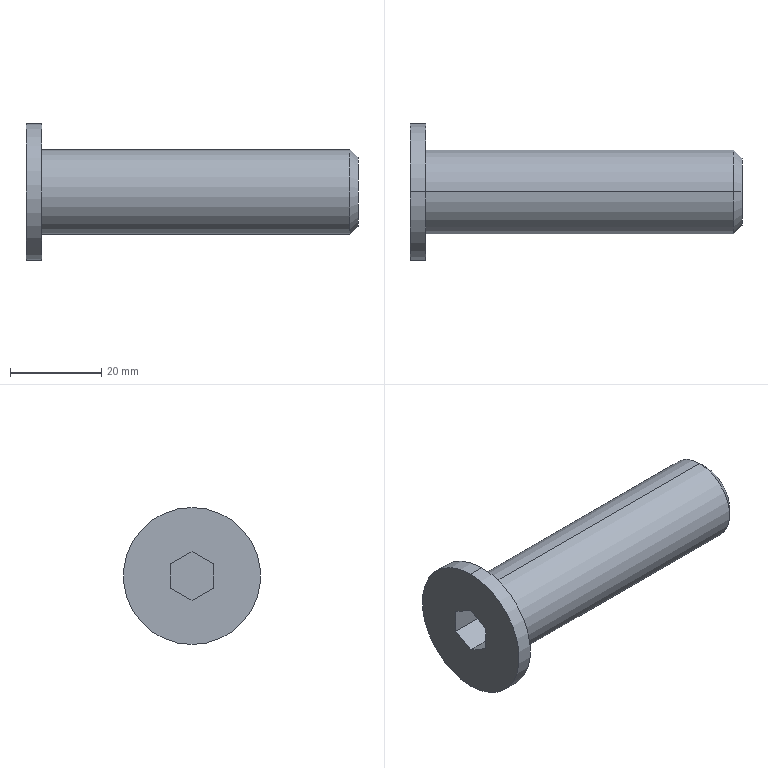Part | SolidWorks | features BaseBody 1 | 1 solid | 16 faces | box 72.692 x 30 x 30 mm | volume 20042 mm3 | plane 10 | cylinder 4 | cone 2 | commonest cylinder face diameters 18.462 x2 30 x2
STEP:
#1=CARTESIAN_POINT('',(-37.408,269.115,278.462));
#2=VERTEX_POINT('',#1);
#3=CARTESIAN_POINT('',(-37.408,269.115,260.));
#4=VERTEX_POINT('',#3);
#5=CARTESIAN_POINT('',(-37.408,269.115,269.231));
#6=DIRECTION('',(-1.,0.,0.));
#7=DIRECTION('',(0.,0.,1.));
#8=AXIS2_PLACEMENT_3D('',#5,#6,#7);
#9=CIRCLE('',#8,9.231);
#10=EDGE_CURVE('',#2,#4,#9,.T.);
#11=ORIENTED_EDGE('',*,*,#10,.T.);
#12=CARTESIAN_POINT('',(-104.869,269.115,260.));
#13=VERTEX_POINT('',#12);
#14=CARTESIAN_POINT('',(-35.638,269.115,260.));
#15=DIRECTION('',(-1.,0.,0.));
#16=VECTOR('',#15,1000.);
#17=LINE('',#14,#16);
#18=EDGE_CURVE('',#4,#13,#17,.T.);
#19=ORIENTED_EDGE('',*,*,#18,.T.);
#20=CARTESIAN_POINT('',(-104.869,269.115,278.462));
#21=VERTEX_POINT('',#20);
#22=CARTESIAN_POINT('',(-104.869,269.115,269.231));
#23=DIRECTION('',(1.,0.,0.));
#24=DIRECTION('',(0.,0.,1.));
#25=AXIS2_PLACEMENT_3D('',#22,#23,#24);
#26=CIRCLE('',#25,9.231);
#27=EDGE_CURVE('',#13,#21,#26,.T.);
#28=ORIENTED_EDGE('',*,*,#27,.T.);
#29=CARTESIAN_POINT('',(-35.638,269.115,278.462));
#30=DIRECTION('',(-1.,0.,0.));
#31=VECTOR('',#30,1000.);
#32=LINE('',#29,#31);
#33=EDGE_CURVE('',#2,#21,#32,.T.);
#34=ORIENTED_EDGE('',*,*,#33,.F.);
#35=EDGE_LOOP('',(#11,#19,#28,#34));
#36=FACE_OUTER_BOUND('',#35,.T.);
#37=CARTESIAN_POINT('',(-35.638,269.115,269.231));
#38=DIRECTION('',(-1.,0.,0.));
#39=DIRECTION('',(0.,0.,1.));
#40=AXIS2_PLACEMENT_3D('',#37,#38,#39);
#41=CYLINDRICAL_SURFACE('',#40,9.231);
#42=ADVANCED_FACE('',(#36),#41,.T.);
#43=CARTESIAN_POINT('',(-35.638,269.115,276.692));
#44=VERTEX_POINT('',#43);
#45=CARTESIAN_POINT('',(-35.638,269.115,261.77));
#46=VERTEX_POINT('',#45);
#47=CARTESIAN_POINT('',(-35.638,269.115,269.231));
#48=DIRECTION('',(-1.,0.,0.));
#49=DIRECTION('',(0.,0.,1.));
#50=AXIS2_PLACEMENT_3D('',#47,#48,#49);
#51=CIRCLE('',#50,7.461);
#52=EDGE_CURVE('',#44,#46,#51,.T.);
#53=ORIENTED_EDGE('',*,*,#52,.T.);
#54=CARTESIAN_POINT('',(-37.408,269.115,260.));
#55=DIRECTION('',(-0.7071,0.,-0.7071));
#56=VECTOR('',#55,1000.);
#57=LINE('',#54,#56);
#58=EDGE_CURVE('',#46,#4,#57,.T.);
#59=ORIENTED_EDGE('',*,*,#58,.T.);
#60=ORIENTED_EDGE('',*,*,#10,.F.);
#61=CARTESIAN_POINT('',(-37.408,269.115,278.462));
#62=DIRECTION('',(-0.7071,0.,0.7071));
#63=VECTOR('',#62,1000.);
#64=LINE('',#61,#63);
#65=EDGE_CURVE('',#44,#2,#64,.T.);
#66=ORIENTED_EDGE('',*,*,#65,.F.);
#67=EDGE_LOOP('',(#53,#59,#60,#66));
#68=FACE_OUTER_BOUND('',#67,.T.);
#69=CARTESIAN_POINT('',(-37.408,269.115,269.231));
#70=DIRECTION('',(-1.,0.,0.));
#71=DIRECTION('',(0.,0.,1.));
#72=AXIS2_PLACEMENT_3D('',#69,#70,#71);
#73=CONICAL_SURFACE('',#72,9.231,0.7854);
#74=ADVANCED_FACE('',(#68),#73,.T.);
#75=CARTESIAN_POINT('',(-104.869,269.115,284.231));
#76=VERTEX_POINT('',#75);
#77=CARTESIAN_POINT('',(-104.869,269.115,254.231));
#78=VERTEX_POINT('',#77);
#79=CARTESIAN_POINT('',(-104.869,269.115,269.231));
#80=DIRECTION('',(-1.,0.,0.));
#81=DIRECTION('',(0.,0.,1.));
#82=AXIS2_PLACEMENT_3D('',#79,#80,#81);
#83=CIRCLE('',#82,15.);
#84=EDGE_CURVE('',#76,#78,#83,.T.);
#85=ORIENTED_EDGE('',*,*,#84,.T.);
#86=CARTESIAN_POINT('',(-108.33,269.115,254.231));
#87=VERTEX_POINT('',#86);
#88=CARTESIAN_POINT('',(-35.638,269.115,254.231));
#89=DIRECTION('',(-1.,0.,0.));
#90=VECTOR('',#89,1000.);
#91=LINE('',#88,#90);
#92=EDGE_CURVE('',#78,#87,#91,.T.);
#93=ORIENTED_EDGE('',*,*,#92,.T.);
#94=CARTESIAN_POINT('',(-108.33,269.115,284.231));
#95=VERTEX_POINT('',#94);
#96=CARTESIAN_POINT('',(-108.33,269.115,269.231));
#97=DIRECTION('',(1.,0.,0.));
#98=DIRECTION('',(0.,0.,1.));
#99=AXIS2_PLACEMENT_3D('',#96,#97,#98);
#100=CIRCLE('',#99,15.);
#101=EDGE_CURVE('',#87,#95,#100,.T.);
#102=ORIENTED_EDGE('',*,*,#101,.T.);
#103=CARTESIAN_POINT('',(-35.638,269.115,284.231));
#104=DIRECTION('',(-1.,0.,0.));
#105=VECTOR('',#104,1000.);
#106=LINE('',#103,#105);
#107=EDGE_CURVE('',#76,#95,#106,.T.);
#108=ORIENTED_EDGE('',*,*,#107,.F.);
#109=EDGE_LOOP('',(#85,#93,#102,#108));
#110=FACE_OUTER_BOUND('',#109,.T.);
#111=CARTESIAN_POINT('',(-35.638,269.115,269.231));
#112=DIRECTION('',(-1.,0.,0.));
#113=DIRECTION('',(0.,0.,1.));
#114=AXIS2_PLACEMENT_3D('',#111,#112,#113);
#115=CYLINDRICAL_SURFACE('',#114,15.);
#116=ADVANCED_FACE('',(#110),#115,.T.);
#117=ORIENTED_EDGE('',*,*,#18,.F.);
#118=CARTESIAN_POINT('',(-37.408,269.115,269.231));
#119=DIRECTION('',(-1.,0.,0.));
#120=DIRECTION('',(0.,0.,1.));
#121=AXIS2_PLACEMENT_3D('',#118,#119,#120);
#122=CIRCLE('',#121,9.231);
#123=EDGE_CURVE('',#4,#2,#122,.T.);
#124=ORIENTED_EDGE('',*,*,#123,.T.);
#125=ORIENTED_EDGE('',*,*,#33,.T.);
#126=CARTESIAN_POINT('',(-104.869,269.115,269.231));
#127=DIRECTION('',(1.,0.,0.));
#128=DIRECTION('',(0.,0.,1.));
#129=AXIS2_PLACEMENT_3D('',#126,#127,#128);
#130=CIRCLE('',#129,9.231);
#131=EDGE_CURVE('',#21,#13,#130,.T.);
#132=ORIENTED_EDGE('',*,*,#131,.T.);
#133=EDGE_LOOP('',(#117,#124,#125,#132));
#134=FACE_OUTER_BOUND('',#133,.T.);
#135=CARTESIAN_POINT('',(-35.638,269.115,269.231));
#136=DIRECTION('',(-1.,0.,0.));
#137=DIRECTION('',(0.,0.,1.));
#138=AXIS2_PLACEMENT_3D('',#135,#136,#137);
#139=CYLINDRICAL_SURFACE('',#138,9.231);
#140=ADVANCED_FACE('',(#134),#139,.T.);
#141=ORIENTED_EDGE('',*,*,#58,.F.);
#142=CARTESIAN_POINT('',(-35.638,269.115,269.231));
#143=DIRECTION('',(-1.,0.,0.));
#144=DIRECTION('',(0.,0.,1.));
#145=AXIS2_PLACEMENT_3D('',#142,#143,#144);
#146=CIRCLE('',#145,7.461);
#147=EDGE_CURVE('',#46,#44,#146,.T.);
#148=ORIENTED_EDGE('',*,*,#147,.T.);
#149=ORIENTED_EDGE('',*,*,#65,.T.);
#150=ORIENTED_EDGE('',*,*,#123,.F.);
#151=EDGE_LOOP('',(#141,#148,#149,#150));
#152=FACE_OUTER_BOUND('',#151,.T.);
#153=CARTESIAN_POINT('',(-37.408,269.115,269.231));
#154=DIRECTION('',(-1.,0.,0.));
#155=DIRECTION('',(0.,0.,1.));
#156=AXIS2_PLACEMENT_3D('',#153,#154,#155);
#157=CONICAL_SURFACE('',#156,9.231,0.7854);
#158=ADVANCED_FACE('',(#152),#157,.T.);
#159=ORIENTED_EDGE('',*,*,#131,.F.);
#160=ORIENTED_EDGE('',*,*,#27,.F.);
#161=EDGE_LOOP('',(#159,#160));
#162=FACE_BOUND('',#161,.T.);
#163=ORIENTED_EDGE('',*,*,#84,.F.);
#164=CARTESIAN_POINT('',(-104.869,269.115,269.231));
#165=DIRECTION('',(-1.,0.,0.));
#166=DIRECTION('',(0.,0.,1.));
#167=AXIS2_PLACEMENT_3D('',#164,#165,#166);
#168=CIRCLE('',#167,15.);
#169=EDGE_CURVE('',#78,#76,#168,.T.);
#170=ORIENTED_EDGE('',*,*,#169,.F.);
#171=EDGE_LOOP('',(#163,#170));
#172=FACE_OUTER_BOUND('',#171,.T.);
#173=CARTESIAN_POINT('',(-104.869,284.115,269.231));
#174=DIRECTION('',(-1.,0.,0.));
#175=DIRECTION('',(0.,0.,1.));
#176=AXIS2_PLACEMENT_3D('',#173,#174,#175);
#177=PLANE('',#176);
#178=ADVANCED_FACE('',(#162,#172),#177,.F.);
#179=ORIENTED_EDGE('',*,*,#52,.F.);
#180=ORIENTED_EDGE('',*,*,#147,.F.);
#181=EDGE_LOOP('',(#179,#180));
#182=FACE_OUTER_BOUND('',#181,.T.);
#183=CARTESIAN_POINT('',(-35.638,276.576,269.231));
#184=DIRECTION('',(-1.,0.,0.));
#185=DIRECTION('',(0.,0.,1.));
#186=AXIS2_PLACEMENT_3D('',#183,#184,#185);
#187=PLANE('',#186);
#188=ADVANCED_FACE('',(#182),#187,.F.);
#189=ORIENTED_EDGE('',*,*,#92,.F.);
#190=ORIENTED_EDGE('',*,*,#169,.T.);
#191=ORIENTED_EDGE('',*,*,#107,.T.);
#192=CARTESIAN_POINT('',(-108.33,269.115,269.231));
#193=DIRECTION('',(1.,0.,0.));
#194=DIRECTION('',(0.,0.,1.));
#195=AXIS2_PLACEMENT_3D('',#192,#193,#194);
#196=CIRCLE('',#195,15.);
#197=EDGE_CURVE('',#95,#87,#196,.T.);
#198=ORIENTED_EDGE('',*,*,#197,.T.);
#199=EDGE_LOOP('',(#189,#190,#191,#198));
#200=FACE_OUTER_BOUND('',#199,.T.);
#201=CARTESIAN_POINT('',(-35.638,269.115,269.231));
#202=DIRECTION('',(-1.,0.,0.));
#203=DIRECTION('',(0.,0.,1.));
#204=AXIS2_PLACEMENT_3D('',#201,#202,#203);
#205=CYLINDRICAL_SURFACE('',#204,15.);
#206=ADVANCED_FACE('',(#200),#205,.T.);
#207=CARTESIAN_POINT('',(-108.33,273.731,271.895));
#208=VERTEX_POINT('',#207);
#209=CARTESIAN_POINT('',(-108.33,273.731,266.566));
#210=VERTEX_POINT('',#209);
#211=CARTESIAN_POINT('',(-108.33,273.731,269.231));
#212=DIRECTION('',(0.,0.,-1.));
#213=VECTOR('',#212,1000.);
#214=LINE('',#211,#213);
#215=EDGE_CURVE('',#208,#210,#214,.T.);
#216=ORIENTED_EDGE('',*,*,#215,.F.);
#217=CARTESIAN_POINT('',(-108.33,269.115,274.56));
#218=VERTEX_POINT('',#217);
#219=CARTESIAN_POINT('',(-108.33,269.115,274.56));
#220=DIRECTION('',(0.,0.866,-0.5));
#221=VECTOR('',#220,1000.);
#222=LINE('',#219,#221);
#223=EDGE_CURVE('',#218,#208,#222,.T.);
#224=ORIENTED_EDGE('',*,*,#223,.F.);
#225=CARTESIAN_POINT('',(-108.33,264.5,271.895));
#226=VERTEX_POINT('',#225);
#227=CARTESIAN_POINT('',(-108.33,264.5,271.895));
#228=DIRECTION('',(0.,0.866,0.5));
#229=VECTOR('',#228,1000.);
#230=LINE('',#227,#229);
#231=EDGE_CURVE('',#226,#218,#230,.T.);
#232=ORIENTED_EDGE('',*,*,#231,.F.);
#233=CARTESIAN_POINT('',(-108.33,264.5,266.566));
#234=VERTEX_POINT('',#233);
#235=CARTESIAN_POINT('',(-108.33,264.5,269.231));
#236=DIRECTION('',(0.,0.,1.));
#237=VECTOR('',#236,1000.);
#238=LINE('',#235,#237);
#239=EDGE_CURVE('',#234,#226,#238,.T.);
#240=ORIENTED_EDGE('',*,*,#239,.F.);
#241=CARTESIAN_POINT('',(-108.33,269.115,263.901));
#242=VERTEX_POINT('',#241);
#243=CARTESIAN_POINT('',(-108.33,269.115,263.901));
#244=DIRECTION('',(0.,-0.866,0.5));
#245=VECTOR('',#244,1000.);
#246=LINE('',#243,#245);
#247=EDGE_CURVE('',#242,#234,#246,.T.);
#248=ORIENTED_EDGE('',*,*,#247,.F.);
#249=CARTESIAN_POINT('',(-108.33,273.731,266.566));
#250=DIRECTION('',(0.,-0.866,-0.5));
#251=VECTOR('',#250,1000.);
#252=LINE('',#249,#251);
#253=EDGE_CURVE('',#210,#242,#252,.T.);
#254=ORIENTED_EDGE('',*,*,#253,.F.);
#255=EDGE_LOOP('',(#216,#224,#232,#240,#248,#254));
#256=FACE_BOUND('',#255,.T.);
#257=ORIENTED_EDGE('',*,*,#197,.F.);
#258=ORIENTED_EDGE('',*,*,#101,.F.);
#259=EDGE_LOOP('',(#257,#258));
#260=FACE_OUTER_BOUND('',#259,.T.);
#261=CARTESIAN_POINT('',(-108.33,269.115,269.231));
#262=DIRECTION('',(1.,0.,0.));
#263=DIRECTION('',(0.,0.,-1.));
#264=AXIS2_PLACEMENT_3D('',#261,#262,#263);
#265=PLANE('',#264);
#266=ADVANCED_FACE('',(#256,#260),#265,.F.);
#267=CARTESIAN_POINT('',(-96.792,269.115,263.901));
#268=VERTEX_POINT('',#267);
#269=CARTESIAN_POINT('',(-96.792,269.115,263.901));
#270=DIRECTION('',(1.,0.,0.));
#271=VECTOR('',#270,1000.);
#272=LINE('',#269,#271);
#273=EDGE_CURVE('',#242,#268,#272,.T.);
#274=ORIENTED_EDGE('',*,*,#273,.T.);
#275=CARTESIAN_POINT('',(-96.792,273.731,266.566));
#276=VERTEX_POINT('',#275);
#277=CARTESIAN_POINT('',(-96.792,269.115,263.901));
#278=DIRECTION('',(0.,0.866,0.5));
#279=VECTOR('',#278,1000.);
#280=LINE('',#277,#279);
#281=EDGE_CURVE('',#268,#276,#280,.T.);
#282=ORIENTED_EDGE('',*,*,#281,.T.);
#283=CARTESIAN_POINT('',(-96.792,273.731,266.566));
#284=DIRECTION('',(-1.,0.,0.));
#285=VECTOR('',#284,1000.);
#286=LINE('',#283,#285);
#287=EDGE_CURVE('',#276,#210,#286,.T.);
#288=ORIENTED_EDGE('',*,*,#287,.T.);
#289=ORIENTED_EDGE('',*,*,#253,.T.);
#290=EDGE_LOOP('',(#274,#282,#288,#289));
#291=FACE_OUTER_BOUND('',#290,.T.);
#292=CARTESIAN_POINT('',(-96.792,269.115,263.901));
#293=DIRECTION('',(0.,-0.5,0.866));
#294=DIRECTION('',(0.,-0.866,-0.5));
#295=AXIS2_PLACEMENT_3D('',#292,#293,#294);
#296=PLANE('',#295);
#297=ADVANCED_FACE('',(#291),#296,.T.);
#298=ORIENTED_EDGE('',*,*,#287,.F.);
#299=CARTESIAN_POINT('',(-96.792,273.731,271.895));
#300=VERTEX_POINT('',#299);
#301=CARTESIAN_POINT('',(-96.792,273.731,266.566));
#302=DIRECTION('',(0.,0.,1.));
#303=VECTOR('',#302,1000.);
#304=LINE('',#301,#303);
#305=EDGE_CURVE('',#276,#300,#304,.T.);
#306=ORIENTED_EDGE('',*,*,#305,.T.);
#307=CARTESIAN_POINT('',(-96.792,273.731,271.895));
#308=DIRECTION('',(-1.,0.,0.));
#309=VECTOR('',#308,1000.);
#310=LINE('',#307,#309);
#311=EDGE_CURVE('',#300,#208,#310,.T.);
#312=ORIENTED_EDGE('',*,*,#311,.T.);
#313=ORIENTED_EDGE('',*,*,#215,.T.);
#314=EDGE_LOOP('',(#298,#306,#312,#313));
#315=FACE_OUTER_BOUND('',#314,.T.);
#316=CARTESIAN_POINT('',(-96.792,273.731,266.566));
#317=DIRECTION('',(0.,-1.,0.));
#318=DIRECTION('',(0.,0.,-1.));
#319=AXIS2_PLACEMENT_3D('',#316,#317,#318);
#320=PLANE('',#319);
#321=ADVANCED_FACE('',(#315),#320,.T.);
#322=ORIENTED_EDGE('',*,*,#311,.F.);
#323=CARTESIAN_POINT('',(-96.792,269.115,274.56));
#324=VERTEX_POINT('',#323);
#325=CARTESIAN_POINT('',(-96.792,273.731,271.895));
#326=DIRECTION('',(0.,-0.866,0.5));
#327=VECTOR('',#326,1000.);
#328=LINE('',#325,#327);
#329=EDGE_CURVE('',#300,#324,#328,.T.);
#330=ORIENTED_EDGE('',*,*,#329,.T.);
#331=CARTESIAN_POINT('',(-96.792,269.115,274.56));
#332=DIRECTION('',(-1.,0.,0.));
#333=VECTOR('',#332,1000.);
#334=LINE('',#331,#333);
#335=EDGE_CURVE('',#324,#218,#334,.T.);
#336=ORIENTED_EDGE('',*,*,#335,.T.);
#337=ORIENTED_EDGE('',*,*,#223,.T.);
#338=EDGE_LOOP('',(#322,#330,#336,#337));
#339=FACE_OUTER_BOUND('',#338,.T.);
#340=CARTESIAN_POINT('',(-96.792,273.731,271.895));
#341=DIRECTION('',(0.,-0.5,-0.866));
#342=DIRECTION('',(0.,0.866,-0.5));
#343=AXIS2_PLACEMENT_3D('',#340,#341,#342);
#344=PLANE('',#343);
#345=ADVANCED_FACE('',(#339),#344,.T.);
#346=ORIENTED_EDGE('',*,*,#335,.F.);
#347=CARTESIAN_POINT('',(-96.792,264.5,271.895));
#348=VERTEX_POINT('',#347);
#349=CARTESIAN_POINT('',(-96.792,269.115,274.56));
#350=DIRECTION('',(0.,-0.866,-0.5));
#351=VECTOR('',#350,1000.);
#352=LINE('',#349,#351);
#353=EDGE_CURVE('',#324,#348,#352,.T.);
#354=ORIENTED_EDGE('',*,*,#353,.T.);
#355=CARTESIAN_POINT('',(-96.792,264.5,271.895));
#356=DIRECTION('',(-1.,0.,0.));
#357=VECTOR('',#356,1000.);
#358=LINE('',#355,#357);
#359=EDGE_CURVE('',#348,#226,#358,.T.);
#360=ORIENTED_EDGE('',*,*,#359,.T.);
#361=ORIENTED_EDGE('',*,*,#231,.T.);
#362=EDGE_LOOP('',(#346,#354,#360,#361));
#363=FACE_OUTER_BOUND('',#362,.T.);
#364=CARTESIAN_POINT('',(-96.792,269.115,274.56));
#365=DIRECTION('',(0.,0.5,-0.866));
#366=DIRECTION('',(0.,0.866,0.5));
#367=AXIS2_PLACEMENT_3D('',#364,#365,#366);
#368=PLANE('',#367);
#369=ADVANCED_FACE('',(#363),#368,.T.);
#370=ORIENTED_EDGE('',*,*,#359,.F.);
#371=CARTESIAN_POINT('',(-96.792,264.5,266.566));
#372=VERTEX_POINT('',#371);
#373=CARTESIAN_POINT('',(-96.792,264.5,271.895));
#374=DIRECTION('',(0.,0.,-1.));
#375=VECTOR('',#374,1000.);
#376=LINE('',#373,#375);
#377=EDGE_CURVE('',#348,#372,#376,.T.);
#378=ORIENTED_EDGE('',*,*,#377,.T.);
#379=CARTESIAN_POINT('',(-96.792,264.5,266.566));
#380=DIRECTION('',(-1.,0.,0.));
#381=VECTOR('',#380,1000.);
#382=LINE('',#379,#381);
#383=EDGE_CURVE('',#372,#234,#382,.T.);
#384=ORIENTED_EDGE('',*,*,#383,.T.);
#385=ORIENTED_EDGE('',*,*,#239,.T.);
#386=EDGE_LOOP('',(#370,#378,#384,#385));
#387=FACE_OUTER_BOUND('',#386,.T.);
#388=CARTESIAN_POINT('',(-96.792,264.5,271.895));
#389=DIRECTION('',(0.,1.,0.));
#390=DIRECTION('',(0.,0.,1.));
#391=AXIS2_PLACEMENT_3D('',#388,#389,#390);
#392=PLANE('',#391);
#393=ADVANCED_FACE('',(#387),#392,.T.);
#394=ORIENTED_EDGE('',*,*,#383,.F.);
#395=CARTESIAN_POINT('',(-96.792,264.5,266.566));
#396=DIRECTION('',(0.,0.866,-0.5));
#397=VECTOR('',#396,1000.);
#398=LINE('',#395,#397);
#399=EDGE_CURVE('',#372,#268,#398,.T.);
#400=ORIENTED_EDGE('',*,*,#399,.T.);
#401=ORIENTED_EDGE('',*,*,#273,.F.);
#402=ORIENTED_EDGE('',*,*,#247,.T.);
#403=EDGE_LOOP('',(#394,#400,#401,#402));
#404=FACE_OUTER_BOUND('',#403,.T.);
#405=CARTESIAN_POINT('',(-96.792,264.5,266.566));
#406=DIRECTION('',(0.,0.5,0.866));
#407=DIRECTION('',(0.,-0.866,0.5));
#408=AXIS2_PLACEMENT_3D('',#405,#406,#407);
#409=PLANE('',#408);
#410=ADVANCED_FACE('',(#404),#409,.T.);
#411=ORIENTED_EDGE('',*,*,#281,.F.);
#412=ORIENTED_EDGE('',*,*,#399,.F.);
#413=ORIENTED_EDGE('',*,*,#377,.F.);
#414=ORIENTED_EDGE('',*,*,#353,.F.);
#415=ORIENTED_EDGE('',*,*,#329,.F.);
#416=ORIENTED_EDGE('',*,*,#305,.F.);
#417=EDGE_LOOP('',(#411,#412,#413,#414,#415,#416));
#418=FACE_OUTER_BOUND('',#417,.T.);
#419=CARTESIAN_POINT('',(-96.792,269.115,269.231));
#420=DIRECTION('',(1.,0.,0.));
#421=DIRECTION('',(0.,0.,-1.));
#422=AXIS2_PLACEMENT_3D('',#419,#420,#421);
#423=PLANE('',#422);
#424=ADVANCED_FACE('',(#418),#423,.F.);
#425=CLOSED_SHELL('',(#42,#74,#116,#140,#158,#178,#188,#206,#266,#297,#321,#345,#369,#393,#410,#424));
#426=MANIFOLD_SOLID_BREP('',#425);
#427=CARTESIAN_POINT('',(0.,0.,0.));
#428=DIRECTION('',(0.,0.,1.));
#429=DIRECTION('',(1.,0.,0.));
#430=AXIS2_PLACEMENT_3D('',#427,#428,#429);
#431=(LENGTH_UNIT()NAMED_UNIT(*)SI_UNIT(.MILLI.,.METRE.));
#432=UNCERTAINTY_MEASURE_WITH_UNIT(LENGTH_MEASURE(0.00001),#431,'','');
#433=(NAMED_UNIT(*)PLANE_ANGLE_UNIT()SI_UNIT($,.RADIAN.));
#434=(NAMED_UNIT(*)SI_UNIT($,.STERADIAN.)SOLID_ANGLE_UNIT());
#435=(GEOMETRIC_REPRESENTATION_CONTEXT(3)GLOBAL_UNCERTAINTY_ASSIGNED_CONTEXT((#432))GLOBAL_UNIT_ASSIGNED_CONTEXT((#431,#433,#434))REPRESENTATION_CONTEXT('',''));
#436=ADVANCED_BREP_SHAPE_REPRESENTATION('',(#426,#430),#435);